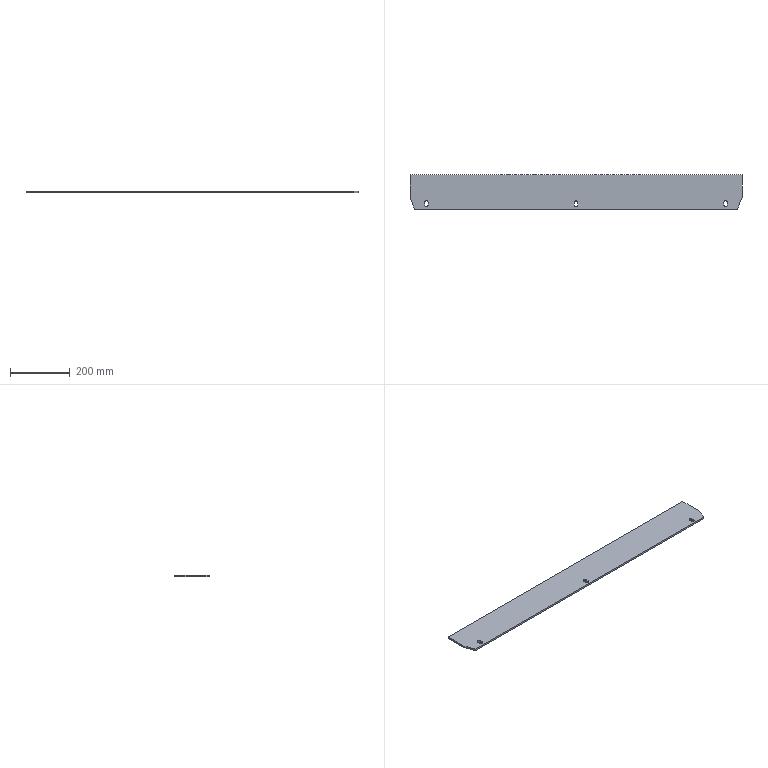Part | SolidWorks | features Extrusion 1, ICE 1 | 1 solid | 20 faces | box 1110 x 115 x 6 mm | volume 758807 mm3 | plane 14 | cylinder 6 | commonest cylinder face diameters 11 x6
STEP:
#1=CARTESIAN_POINT('',(-555.,57.5,0.));
#2=VERTEX_POINT('',#1);
#3=CARTESIAN_POINT('',(-555.,-17.5,0.));
#4=VERTEX_POINT('',#3);
#5=CARTESIAN_POINT('',(-555.,-57.5,0.));
#6=DIRECTION('',(0.,-1.,0.));
#7=VECTOR('',#6,1000.);
#8=LINE('',#5,#7);
#9=EDGE_CURVE('',#2,#4,#8,.T.);
#10=ORIENTED_EDGE('',*,*,#9,.T.);
#11=CARTESIAN_POINT('',(-555.,-17.5,6.));
#12=VERTEX_POINT('',#11);
#13=CARTESIAN_POINT('',(-555.,-17.5,0.));
#14=DIRECTION('',(0.,0.,1.));
#15=VECTOR('',#14,1000.);
#16=LINE('',#13,#15);
#17=EDGE_CURVE('',#4,#12,#16,.T.);
#18=ORIENTED_EDGE('',*,*,#17,.T.);
#19=CARTESIAN_POINT('',(-555.,57.5,6.));
#20=VERTEX_POINT('',#19);
#21=CARTESIAN_POINT('',(-555.,-57.5,6.));
#22=DIRECTION('',(0.,-1.,0.));
#23=VECTOR('',#22,1000.);
#24=LINE('',#21,#23);
#25=EDGE_CURVE('',#20,#12,#24,.T.);
#26=ORIENTED_EDGE('',*,*,#25,.F.);
#27=CARTESIAN_POINT('',(-555.,57.5,6.));
#28=DIRECTION('',(0.,0.,-1.));
#29=VECTOR('',#28,1000.);
#30=LINE('',#27,#29);
#31=EDGE_CURVE('',#20,#2,#30,.T.);
#32=ORIENTED_EDGE('',*,*,#31,.T.);
#33=EDGE_LOOP('',(#10,#18,#26,#32));
#34=FACE_OUTER_BOUND('',#33,.T.);
#35=CARTESIAN_POINT('',(-555.,-57.5,6.));
#36=DIRECTION('',(1.,0.,0.));
#37=DIRECTION('',(0.,0.,-1.));
#38=AXIS2_PLACEMENT_3D('',#35,#36,#37);
#39=PLANE('',#38);
#40=ADVANCED_FACE('',(#34),#39,.F.);
#41=CARTESIAN_POINT('',(-540.,-57.5,6.));
#42=VERTEX_POINT('',#41);
#43=CARTESIAN_POINT('',(540.,-57.5,6.));
#44=VERTEX_POINT('',#43);
#45=CARTESIAN_POINT('',(555.,-57.5,6.));
#46=DIRECTION('',(1.,0.,0.));
#47=VECTOR('',#46,1000.);
#48=LINE('',#45,#47);
#49=EDGE_CURVE('',#42,#44,#48,.T.);
#50=ORIENTED_EDGE('',*,*,#49,.F.);
#51=CARTESIAN_POINT('',(-540.,-57.5,0.));
#52=VERTEX_POINT('',#51);
#53=CARTESIAN_POINT('',(-540.,-57.5,0.));
#54=DIRECTION('',(0.,0.,1.));
#55=VECTOR('',#54,1000.);
#56=LINE('',#53,#55);
#57=EDGE_CURVE('',#52,#42,#56,.T.);
#58=ORIENTED_EDGE('',*,*,#57,.F.);
#59=CARTESIAN_POINT('',(540.,-57.5,0.));
#60=VERTEX_POINT('',#59);
#61=CARTESIAN_POINT('',(555.,-57.5,0.));
#62=DIRECTION('',(1.,0.,0.));
#63=VECTOR('',#62,1000.);
#64=LINE('',#61,#63);
#65=EDGE_CURVE('',#52,#60,#64,.T.);
#66=ORIENTED_EDGE('',*,*,#65,.T.);
#67=CARTESIAN_POINT('',(540.,-57.5,0.));
#68=DIRECTION('',(0.,0.,1.));
#69=VECTOR('',#68,1000.);
#70=LINE('',#67,#69);
#71=EDGE_CURVE('',#60,#44,#70,.T.);
#72=ORIENTED_EDGE('',*,*,#71,.T.);
#73=EDGE_LOOP('',(#50,#58,#66,#72));
#74=FACE_OUTER_BOUND('',#73,.T.);
#75=CARTESIAN_POINT('',(555.,-57.5,6.));
#76=DIRECTION('',(0.,1.,0.));
#77=DIRECTION('',(-1.,0.,0.));
#78=AXIS2_PLACEMENT_3D('',#75,#76,#77);
#79=PLANE('',#78);
#80=ADVANCED_FACE('',(#74),#79,.F.);
#81=CARTESIAN_POINT('',(555.,-17.5,6.));
#82=VERTEX_POINT('',#81);
#83=CARTESIAN_POINT('',(555.,57.5,6.));
#84=VERTEX_POINT('',#83);
#85=CARTESIAN_POINT('',(555.,-57.5,6.));
#86=DIRECTION('',(0.,1.,0.));
#87=VECTOR('',#86,1000.);
#88=LINE('',#85,#87);
#89=EDGE_CURVE('',#82,#84,#88,.T.);
#90=ORIENTED_EDGE('',*,*,#89,.F.);
#91=CARTESIAN_POINT('',(555.,-17.5,0.));
#92=VERTEX_POINT('',#91);
#93=CARTESIAN_POINT('',(555.,-17.5,0.));
#94=DIRECTION('',(0.,0.,1.));
#95=VECTOR('',#94,1000.);
#96=LINE('',#93,#95);
#97=EDGE_CURVE('',#92,#82,#96,.T.);
#98=ORIENTED_EDGE('',*,*,#97,.F.);
#99=CARTESIAN_POINT('',(555.,57.5,0.));
#100=VERTEX_POINT('',#99);
#101=CARTESIAN_POINT('',(555.,-57.5,0.));
#102=DIRECTION('',(0.,1.,0.));
#103=VECTOR('',#102,1000.);
#104=LINE('',#101,#103);
#105=EDGE_CURVE('',#92,#100,#104,.T.);
#106=ORIENTED_EDGE('',*,*,#105,.T.);
#107=CARTESIAN_POINT('',(555.,57.5,6.));
#108=DIRECTION('',(0.,0.,-1.));
#109=VECTOR('',#108,1000.);
#110=LINE('',#107,#109);
#111=EDGE_CURVE('',#84,#100,#110,.T.);
#112=ORIENTED_EDGE('',*,*,#111,.F.);
#113=EDGE_LOOP('',(#90,#98,#106,#112));
#114=FACE_OUTER_BOUND('',#113,.T.);
#115=CARTESIAN_POINT('',(555.,-57.5,6.));
#116=DIRECTION('',(-1.,0.,0.));
#117=DIRECTION('',(0.,0.,1.));
#118=AXIS2_PLACEMENT_3D('',#115,#116,#117);
#119=PLANE('',#118);
#120=ADVANCED_FACE('',(#114),#119,.F.);
#121=CARTESIAN_POINT('',(555.,57.5,0.));
#122=DIRECTION('',(-1.,0.,0.));
#123=VECTOR('',#122,1000.);
#124=LINE('',#121,#123);
#125=EDGE_CURVE('',#100,#2,#124,.T.);
#126=ORIENTED_EDGE('',*,*,#125,.T.);
#127=ORIENTED_EDGE('',*,*,#31,.F.);
#128=CARTESIAN_POINT('',(555.,57.5,6.));
#129=DIRECTION('',(-1.,0.,0.));
#130=VECTOR('',#129,1000.);
#131=LINE('',#128,#130);
#132=EDGE_CURVE('',#84,#20,#131,.T.);
#133=ORIENTED_EDGE('',*,*,#132,.F.);
#134=ORIENTED_EDGE('',*,*,#111,.T.);
#135=EDGE_LOOP('',(#126,#127,#133,#134));
#136=FACE_OUTER_BOUND('',#135,.T.);
#137=CARTESIAN_POINT('',(555.,57.5,6.));
#138=DIRECTION('',(0.,-1.,0.));
#139=DIRECTION('',(1.,0.,0.));
#140=AXIS2_PLACEMENT_3D('',#137,#138,#139);
#141=PLANE('',#140);
#142=ADVANCED_FACE('',(#136),#141,.F.);
#143=CARTESIAN_POINT('',(5.5,-35.,6.));
#144=VERTEX_POINT('',#143);
#145=CARTESIAN_POINT('',(-5.5,-35.,6.));
#146=VERTEX_POINT('',#145);
#147=CARTESIAN_POINT('',(0.,-35.,6.));
#148=DIRECTION('',(0.,0.,1.));
#149=DIRECTION('',(1.,0.,0.));
#150=AXIS2_PLACEMENT_3D('',#147,#148,#149);
#151=CIRCLE('',#150,5.5);
#152=EDGE_CURVE('',#144,#146,#151,.T.);
#153=ORIENTED_EDGE('',*,*,#152,.F.);
#154=CARTESIAN_POINT('',(5.5,-44.,6.));
#155=VERTEX_POINT('',#154);
#156=CARTESIAN_POINT('',(5.5,-35.,6.));
#157=DIRECTION('',(0.,1.,0.));
#158=VECTOR('',#157,1000.);
#159=LINE('',#156,#158);
#160=EDGE_CURVE('',#155,#144,#159,.T.);
#161=ORIENTED_EDGE('',*,*,#160,.F.);
#162=CARTESIAN_POINT('',(-5.5,-44.,6.));
#163=VERTEX_POINT('',#162);
#164=CARTESIAN_POINT('',(0.,-44.,6.));
#165=DIRECTION('',(0.,0.,1.));
#166=DIRECTION('',(1.,0.,0.));
#167=AXIS2_PLACEMENT_3D('',#164,#165,#166);
#168=CIRCLE('',#167,5.5);
#169=EDGE_CURVE('',#163,#155,#168,.T.);
#170=ORIENTED_EDGE('',*,*,#169,.F.);
#171=CARTESIAN_POINT('',(-5.5,-35.,6.));
#172=DIRECTION('',(0.,-1.,0.));
#173=VECTOR('',#172,1000.);
#174=LINE('',#171,#173);
#175=EDGE_CURVE('',#146,#163,#174,.T.);
#176=ORIENTED_EDGE('',*,*,#175,.F.);
#177=EDGE_LOOP('',(#153,#161,#170,#176));
#178=FACE_BOUND('',#177,.T.);
#179=CARTESIAN_POINT('',(494.5,-44.,6.));
#180=VERTEX_POINT('',#179);
#181=CARTESIAN_POINT('',(505.5,-44.,6.));
#182=VERTEX_POINT('',#181);
#183=CARTESIAN_POINT('',(500.,-44.,6.));
#184=DIRECTION('',(0.,0.,1.));
#185=DIRECTION('',(1.,0.,0.));
#186=AXIS2_PLACEMENT_3D('',#183,#184,#185);
#187=CIRCLE('',#186,5.5);
#188=EDGE_CURVE('',#180,#182,#187,.T.);
#189=ORIENTED_EDGE('',*,*,#188,.F.);
#190=CARTESIAN_POINT('',(494.5,-35.,6.));
#191=VERTEX_POINT('',#190);
#192=CARTESIAN_POINT('',(494.5,-44.,6.));
#193=DIRECTION('',(0.,-1.,0.));
#194=VECTOR('',#193,1000.);
#195=LINE('',#192,#194);
#196=EDGE_CURVE('',#191,#180,#195,.T.);
#197=ORIENTED_EDGE('',*,*,#196,.F.);
#198=CARTESIAN_POINT('',(505.5,-35.,6.));
#199=VERTEX_POINT('',#198);
#200=CARTESIAN_POINT('',(500.,-35.,6.));
#201=DIRECTION('',(0.,0.,1.));
#202=DIRECTION('',(1.,0.,0.));
#203=AXIS2_PLACEMENT_3D('',#200,#201,#202);
#204=CIRCLE('',#203,5.5);
#205=EDGE_CURVE('',#199,#191,#204,.T.);
#206=ORIENTED_EDGE('',*,*,#205,.F.);
#207=CARTESIAN_POINT('',(505.5,-44.,6.));
#208=DIRECTION('',(0.,1.,0.));
#209=VECTOR('',#208,1000.);
#210=LINE('',#207,#209);
#211=EDGE_CURVE('',#182,#199,#210,.T.);
#212=ORIENTED_EDGE('',*,*,#211,.F.);
#213=EDGE_LOOP('',(#189,#197,#206,#212));
#214=FACE_BOUND('',#213,.T.);
#215=CARTESIAN_POINT('',(-555.,-17.5,6.));
#216=DIRECTION('',(-0.3511,0.9363,0.));
#217=VECTOR('',#216,1000.);
#218=LINE('',#215,#217);
#219=EDGE_CURVE('',#42,#12,#218,.T.);
#220=ORIENTED_EDGE('',*,*,#219,.F.);
#221=ORIENTED_EDGE('',*,*,#49,.T.);
#222=CARTESIAN_POINT('',(555.,-17.5,6.));
#223=DIRECTION('',(-0.3511,-0.9363,0.));
#224=VECTOR('',#223,1000.);
#225=LINE('',#222,#224);
#226=EDGE_CURVE('',#82,#44,#225,.T.);
#227=ORIENTED_EDGE('',*,*,#226,.F.);
#228=ORIENTED_EDGE('',*,*,#89,.T.);
#229=ORIENTED_EDGE('',*,*,#132,.T.);
#230=ORIENTED_EDGE('',*,*,#25,.T.);
#231=EDGE_LOOP('',(#220,#221,#227,#228,#229,#230));
#232=FACE_OUTER_BOUND('',#231,.T.);
#233=CARTESIAN_POINT('',(-494.5,-35.,6.));
#234=VERTEX_POINT('',#233);
#235=CARTESIAN_POINT('',(-505.5,-35.,6.));
#236=VERTEX_POINT('',#235);
#237=CARTESIAN_POINT('',(-500.,-35.,6.));
#238=DIRECTION('',(0.,0.,1.));
#239=DIRECTION('',(1.,0.,0.));
#240=AXIS2_PLACEMENT_3D('',#237,#238,#239);
#241=CIRCLE('',#240,5.5);
#242=EDGE_CURVE('',#234,#236,#241,.T.);
#243=ORIENTED_EDGE('',*,*,#242,.F.);
#244=CARTESIAN_POINT('',(-494.5,-44.,6.));
#245=VERTEX_POINT('',#244);
#246=CARTESIAN_POINT('',(-494.5,-35.,6.));
#247=DIRECTION('',(0.,1.,0.));
#248=VECTOR('',#247,1000.);
#249=LINE('',#246,#248);
#250=EDGE_CURVE('',#245,#234,#249,.T.);
#251=ORIENTED_EDGE('',*,*,#250,.F.);
#252=CARTESIAN_POINT('',(-505.5,-44.,6.));
#253=VERTEX_POINT('',#252);
#254=CARTESIAN_POINT('',(-500.,-44.,6.));
#255=DIRECTION('',(0.,0.,1.));
#256=DIRECTION('',(1.,0.,0.));
#257=AXIS2_PLACEMENT_3D('',#254,#255,#256);
#258=CIRCLE('',#257,5.5);
#259=EDGE_CURVE('',#253,#245,#258,.T.);
#260=ORIENTED_EDGE('',*,*,#259,.F.);
#261=CARTESIAN_POINT('',(-505.5,-35.,6.));
#262=DIRECTION('',(0.,-1.,0.));
#263=VECTOR('',#262,1000.);
#264=LINE('',#261,#263);
#265=EDGE_CURVE('',#236,#253,#264,.T.);
#266=ORIENTED_EDGE('',*,*,#265,.F.);
#267=EDGE_LOOP('',(#243,#251,#260,#266));
#268=FACE_BOUND('',#267,.T.);
#269=CARTESIAN_POINT('',(0.,0.,6.));
#270=DIRECTION('',(0.,0.,1.));
#271=DIRECTION('',(1.,0.,0.));
#272=AXIS2_PLACEMENT_3D('',#269,#270,#271);
#273=PLANE('',#272);
#274=ADVANCED_FACE('',(#178,#214,#232,#268),#273,.T.);
#275=CARTESIAN_POINT('',(5.5,-44.,0.));
#276=VERTEX_POINT('',#275);
#277=CARTESIAN_POINT('',(5.5,-35.,0.));
#278=VERTEX_POINT('',#277);
#279=CARTESIAN_POINT('',(5.5,-35.,0.));
#280=DIRECTION('',(0.,1.,0.));
#281=VECTOR('',#280,1000.);
#282=LINE('',#279,#281);
#283=EDGE_CURVE('',#276,#278,#282,.T.);
#284=ORIENTED_EDGE('',*,*,#283,.T.);
#285=CARTESIAN_POINT('',(-5.5,-35.,0.));
#286=VERTEX_POINT('',#285);
#287=CARTESIAN_POINT('',(0.,-35.,0.));
#288=DIRECTION('',(0.,0.,1.));
#289=DIRECTION('',(1.,0.,0.));
#290=AXIS2_PLACEMENT_3D('',#287,#288,#289);
#291=CIRCLE('',#290,5.5);
#292=EDGE_CURVE('',#278,#286,#291,.T.);
#293=ORIENTED_EDGE('',*,*,#292,.T.);
#294=CARTESIAN_POINT('',(-5.5,-44.,0.));
#295=VERTEX_POINT('',#294);
#296=CARTESIAN_POINT('',(-5.5,-35.,0.));
#297=DIRECTION('',(0.,-1.,0.));
#298=VECTOR('',#297,1000.);
#299=LINE('',#296,#298);
#300=EDGE_CURVE('',#286,#295,#299,.T.);
#301=ORIENTED_EDGE('',*,*,#300,.T.);
#302=CARTESIAN_POINT('',(0.,-44.,0.));
#303=DIRECTION('',(0.,0.,1.));
#304=DIRECTION('',(1.,0.,0.));
#305=AXIS2_PLACEMENT_3D('',#302,#303,#304);
#306=CIRCLE('',#305,5.5);
#307=EDGE_CURVE('',#295,#276,#306,.T.);
#308=ORIENTED_EDGE('',*,*,#307,.T.);
#309=EDGE_LOOP('',(#284,#293,#301,#308));
#310=FACE_BOUND('',#309,.T.);
#311=CARTESIAN_POINT('',(494.5,-35.,0.));
#312=VERTEX_POINT('',#311);
#313=CARTESIAN_POINT('',(494.5,-44.,0.));
#314=VERTEX_POINT('',#313);
#315=CARTESIAN_POINT('',(494.5,-44.,0.));
#316=DIRECTION('',(0.,-1.,0.));
#317=VECTOR('',#316,1000.);
#318=LINE('',#315,#317);
#319=EDGE_CURVE('',#312,#314,#318,.T.);
#320=ORIENTED_EDGE('',*,*,#319,.T.);
#321=CARTESIAN_POINT('',(505.5,-44.,0.));
#322=VERTEX_POINT('',#321);
#323=CARTESIAN_POINT('',(500.,-44.,0.));
#324=DIRECTION('',(0.,0.,1.));
#325=DIRECTION('',(1.,0.,0.));
#326=AXIS2_PLACEMENT_3D('',#323,#324,#325);
#327=CIRCLE('',#326,5.5);
#328=EDGE_CURVE('',#314,#322,#327,.T.);
#329=ORIENTED_EDGE('',*,*,#328,.T.);
#330=CARTESIAN_POINT('',(505.5,-35.,0.));
#331=VERTEX_POINT('',#330);
#332=CARTESIAN_POINT('',(505.5,-44.,0.));
#333=DIRECTION('',(0.,1.,0.));
#334=VECTOR('',#333,1000.);
#335=LINE('',#332,#334);
#336=EDGE_CURVE('',#322,#331,#335,.T.);
#337=ORIENTED_EDGE('',*,*,#336,.T.);
#338=CARTESIAN_POINT('',(500.,-35.,0.));
#339=DIRECTION('',(0.,0.,1.));
#340=DIRECTION('',(1.,0.,0.));
#341=AXIS2_PLACEMENT_3D('',#338,#339,#340);
#342=CIRCLE('',#341,5.5);
#343=EDGE_CURVE('',#331,#312,#342,.T.);
#344=ORIENTED_EDGE('',*,*,#343,.T.);
#345=EDGE_LOOP('',(#320,#329,#337,#344));
#346=FACE_BOUND('',#345,.T.);
#347=CARTESIAN_POINT('',(-494.5,-44.,0.));
#348=VERTEX_POINT('',#347);
#349=CARTESIAN_POINT('',(-494.5,-35.,0.));
#350=VERTEX_POINT('',#349);
#351=CARTESIAN_POINT('',(-494.5,-35.,0.));
#352=DIRECTION('',(0.,1.,0.));
#353=VECTOR('',#352,1000.);
#354=LINE('',#351,#353);
#355=EDGE_CURVE('',#348,#350,#354,.T.);
#356=ORIENTED_EDGE('',*,*,#355,.T.);
#357=CARTESIAN_POINT('',(-505.5,-35.,0.));
#358=VERTEX_POINT('',#357);
#359=CARTESIAN_POINT('',(-500.,-35.,0.));
#360=DIRECTION('',(0.,0.,1.));
#361=DIRECTION('',(1.,0.,0.));
#362=AXIS2_PLACEMENT_3D('',#359,#360,#361);
#363=CIRCLE('',#362,5.5);
#364=EDGE_CURVE('',#350,#358,#363,.T.);
#365=ORIENTED_EDGE('',*,*,#364,.T.);
#366=CARTESIAN_POINT('',(-505.5,-44.,0.));
#367=VERTEX_POINT('',#366);
#368=CARTESIAN_POINT('',(-505.5,-35.,0.));
#369=DIRECTION('',(0.,-1.,0.));
#370=VECTOR('',#369,1000.);
#371=LINE('',#368,#370);
#372=EDGE_CURVE('',#358,#367,#371,.T.);
#373=ORIENTED_EDGE('',*,*,#372,.T.);
#374=CARTESIAN_POINT('',(-500.,-44.,0.));
#375=DIRECTION('',(0.,0.,1.));
#376=DIRECTION('',(1.,0.,0.));
#377=AXIS2_PLACEMENT_3D('',#374,#375,#376);
#378=CIRCLE('',#377,5.5);
#379=EDGE_CURVE('',#367,#348,#378,.T.);
#380=ORIENTED_EDGE('',*,*,#379,.T.);
#381=EDGE_LOOP('',(#356,#365,#373,#380));
#382=FACE_BOUND('',#381,.T.);
#383=ORIENTED_EDGE('',*,*,#65,.F.);
#384=CARTESIAN_POINT('',(-555.,-17.5,0.));
#385=DIRECTION('',(-0.3511,0.9363,0.));
#386=VECTOR('',#385,1000.);
#387=LINE('',#384,#386);
#388=EDGE_CURVE('',#52,#4,#387,.T.);
#389=ORIENTED_EDGE('',*,*,#388,.T.);
#390=ORIENTED_EDGE('',*,*,#9,.F.);
#391=ORIENTED_EDGE('',*,*,#125,.F.);
#392=ORIENTED_EDGE('',*,*,#105,.F.);
#393=CARTESIAN_POINT('',(555.,-17.5,0.));
#394=DIRECTION('',(-0.3511,-0.9363,0.));
#395=VECTOR('',#394,1000.);
#396=LINE('',#393,#395);
#397=EDGE_CURVE('',#92,#60,#396,.T.);
#398=ORIENTED_EDGE('',*,*,#397,.T.);
#399=EDGE_LOOP('',(#383,#389,#390,#391,#392,#398));
#400=FACE_OUTER_BOUND('',#399,.T.);
#401=CARTESIAN_POINT('',(0.,0.,0.));
#402=DIRECTION('',(0.,0.,1.));
#403=DIRECTION('',(1.,0.,0.));
#404=AXIS2_PLACEMENT_3D('',#401,#402,#403);
#405=PLANE('',#404);
#406=ADVANCED_FACE('',(#310,#346,#382,#400),#405,.F.);
#407=ORIENTED_EDGE('',*,*,#242,.T.);
#408=CARTESIAN_POINT('',(-505.5,-35.,0.));
#409=DIRECTION('',(0.,0.,1.));
#410=VECTOR('',#409,1000.);
#411=LINE('',#408,#410);
#412=EDGE_CURVE('',#358,#236,#411,.T.);
#413=ORIENTED_EDGE('',*,*,#412,.F.);
#414=ORIENTED_EDGE('',*,*,#364,.F.);
#415=CARTESIAN_POINT('',(-494.5,-35.,0.));
#416=DIRECTION('',(0.,0.,1.));
#417=VECTOR('',#416,1000.);
#418=LINE('',#415,#417);
#419=EDGE_CURVE('',#350,#234,#418,.T.);
#420=ORIENTED_EDGE('',*,*,#419,.T.);
#421=EDGE_LOOP('',(#407,#413,#414,#420));
#422=FACE_OUTER_BOUND('',#421,.T.);
#423=CARTESIAN_POINT('',(-500.,-35.,0.));
#424=DIRECTION('',(0.,0.,1.));
#425=DIRECTION('',(1.,0.,0.));
#426=AXIS2_PLACEMENT_3D('',#423,#424,#425);
#427=CYLINDRICAL_SURFACE('',#426,5.5);
#428=ADVANCED_FACE('',(#422),#427,.F.);
#429=ORIENTED_EDGE('',*,*,#250,.T.);
#430=ORIENTED_EDGE('',*,*,#419,.F.);
#431=ORIENTED_EDGE('',*,*,#355,.F.);
#432=CARTESIAN_POINT('',(-494.5,-44.,0.));
#433=DIRECTION('',(0.,0.,1.));
#434=VECTOR('',#433,1000.);
#435=LINE('',#432,#434);
#436=EDGE_CURVE('',#348,#245,#435,.T.);
#437=ORIENTED_EDGE('',*,*,#436,.T.);
#438=EDGE_LOOP('',(#429,#430,#431,#437));
#439=FACE_OUTER_BOUND('',#438,.T.);
#440=CARTESIAN_POINT('',(-494.5,-35.,0.));
#441=DIRECTION('',(1.,0.,0.));
#442=DIRECTION('',(0.,0.,-1.));
#443=AXIS2_PLACEMENT_3D('',#440,#441,#442);
#444=PLANE('',#443);
#445=ADVANCED_FACE('',(#439),#444,.F.);
#446=ORIENTED_EDGE('',*,*,#259,.T.);
#447=ORIENTED_EDGE('',*,*,#436,.F.);
#448=ORIENTED_EDGE('',*,*,#379,.F.);
#449=CARTESIAN_POINT('',(-505.5,-44.,0.));
#450=DIRECTION('',(0.,0.,1.));
#451=VECTOR('',#450,1000.);
#452=LINE('',#449,#451);
#453=EDGE_CURVE('',#367,#253,#452,.T.);
#454=ORIENTED_EDGE('',*,*,#453,.T.);
#455=EDGE_LOOP('',(#446,#447,#448,#454));
#456=FACE_OUTER_BOUND('',#455,.T.);
#457=CARTESIAN_POINT('',(-500.,-44.,0.));
#458=DIRECTION('',(0.,0.,1.));
#459=DIRECTION('',(1.,0.,0.));
#460=AXIS2_PLACEMENT_3D('',#457,#458,#459);
#461=CYLINDRICAL_SURFACE('',#460,5.5);
#462=ADVANCED_FACE('',(#456),#461,.F.);
#463=ORIENTED_EDGE('',*,*,#265,.T.);
#464=ORIENTED_EDGE('',*,*,#453,.F.);
#465=ORIENTED_EDGE('',*,*,#372,.F.);
#466=ORIENTED_EDGE('',*,*,#412,.T.);
#467=EDGE_LOOP('',(#463,#464,#465,#466));
#468=FACE_OUTER_BOUND('',#467,.T.);
#469=CARTESIAN_POINT('',(-505.5,-35.,0.));
#470=DIRECTION('',(-1.,0.,0.));
#471=DIRECTION('',(0.,0.,1.));
#472=AXIS2_PLACEMENT_3D('',#469,#470,#471);
#473=PLANE('',#472);
#474=ADVANCED_FACE('',(#468),#473,.F.);
#475=ORIENTED_EDGE('',*,*,#226,.T.);
#476=ORIENTED_EDGE('',*,*,#71,.F.);
#477=ORIENTED_EDGE('',*,*,#397,.F.);
#478=ORIENTED_EDGE('',*,*,#97,.T.);
#479=EDGE_LOOP('',(#475,#476,#477,#478));
#480=FACE_OUTER_BOUND('',#479,.T.);
#481=CARTESIAN_POINT('',(555.,-17.5,0.));
#482=DIRECTION('',(-0.9363,0.3511,0.));
#483=DIRECTION('',(-0.3511,-0.9363,0.));
#484=AXIS2_PLACEMENT_3D('',#481,#482,#483);
#485=PLANE('',#484);
#486=ADVANCED_FACE('',(#480),#485,.F.);
#487=ORIENTED_EDGE('',*,*,#219,.T.);
#488=ORIENTED_EDGE('',*,*,#17,.F.);
#489=ORIENTED_EDGE('',*,*,#388,.F.);
#490=ORIENTED_EDGE('',*,*,#57,.T.);
#491=EDGE_LOOP('',(#487,#488,#489,#490));
#492=FACE_OUTER_BOUND('',#491,.T.);
#493=CARTESIAN_POINT('',(-555.,-17.5,0.));
#494=DIRECTION('',(0.9363,0.3511,0.));
#495=DIRECTION('',(-0.3511,0.9363,0.));
#496=AXIS2_PLACEMENT_3D('',#493,#494,#495);
#497=PLANE('',#496);
#498=ADVANCED_FACE('',(#492),#497,.F.);
#499=ORIENTED_EDGE('',*,*,#188,.T.);
#500=CARTESIAN_POINT('',(505.5,-44.,0.));
#501=DIRECTION('',(0.,0.,1.));
#502=VECTOR('',#501,1000.);
#503=LINE('',#500,#502);
#504=EDGE_CURVE('',#322,#182,#503,.T.);
#505=ORIENTED_EDGE('',*,*,#504,.F.);
#506=ORIENTED_EDGE('',*,*,#328,.F.);
#507=CARTESIAN_POINT('',(494.5,-44.,0.));
#508=DIRECTION('',(0.,0.,1.));
#509=VECTOR('',#508,1000.);
#510=LINE('',#507,#509);
#511=EDGE_CURVE('',#314,#180,#510,.T.);
#512=ORIENTED_EDGE('',*,*,#511,.T.);
#513=EDGE_LOOP('',(#499,#505,#506,#512));
#514=FACE_OUTER_BOUND('',#513,.T.);
#515=CARTESIAN_POINT('',(500.,-44.,0.));
#516=DIRECTION('',(0.,0.,1.));
#517=DIRECTION('',(1.,0.,0.));
#518=AXIS2_PLACEMENT_3D('',#515,#516,#517);
#519=CYLINDRICAL_SURFACE('',#518,5.5);
#520=ADVANCED_FACE('',(#514),#519,.F.);
#521=ORIENTED_EDGE('',*,*,#196,.T.);
#522=ORIENTED_EDGE('',*,*,#511,.F.);
#523=ORIENTED_EDGE('',*,*,#319,.F.);
#524=CARTESIAN_POINT('',(494.5,-35.,0.));
#525=DIRECTION('',(0.,0.,1.));
#526=VECTOR('',#525,1000.);
#527=LINE('',#524,#526);
#528=EDGE_CURVE('',#312,#191,#527,.T.);
#529=ORIENTED_EDGE('',*,*,#528,.T.);
#530=EDGE_LOOP('',(#521,#522,#523,#529));
#531=FACE_OUTER_BOUND('',#530,.T.);
#532=CARTESIAN_POINT('',(494.5,-44.,0.));
#533=DIRECTION('',(-1.,0.,0.));
#534=DIRECTION('',(0.,0.,1.));
#535=AXIS2_PLACEMENT_3D('',#532,#533,#534);
#536=PLANE('',#535);
#537=ADVANCED_FACE('',(#531),#536,.F.);
#538=ORIENTED_EDGE('',*,*,#205,.T.);
#539=ORIENTED_EDGE('',*,*,#528,.F.);
#540=ORIENTED_EDGE('',*,*,#343,.F.);
#541=CARTESIAN_POINT('',(505.5,-35.,0.));
#542=DIRECTION('',(0.,0.,1.));
#543=VECTOR('',#542,1000.);
#544=LINE('',#541,#543);
#545=EDGE_CURVE('',#331,#199,#544,.T.);
#546=ORIENTED_EDGE('',*,*,#545,.T.);
#547=EDGE_LOOP('',(#538,#539,#540,#546));
#548=FACE_OUTER_BOUND('',#547,.T.);
#549=CARTESIAN_POINT('',(500.,-35.,0.));
#550=DIRECTION('',(0.,0.,1.));
#551=DIRECTION('',(1.,0.,0.));
#552=AXIS2_PLACEMENT_3D('',#549,#550,#551);
#553=CYLINDRICAL_SURFACE('',#552,5.5);
#554=ADVANCED_FACE('',(#548),#553,.F.);
#555=ORIENTED_EDGE('',*,*,#211,.T.);
#556=ORIENTED_EDGE('',*,*,#545,.F.);
#557=ORIENTED_EDGE('',*,*,#336,.F.);
#558=ORIENTED_EDGE('',*,*,#504,.T.);
#559=EDGE_LOOP('',(#555,#556,#557,#558));
#560=FACE_OUTER_BOUND('',#559,.T.);
#561=CARTESIAN_POINT('',(505.5,-44.,0.));
#562=DIRECTION('',(1.,0.,0.));
#563=DIRECTION('',(0.,0.,-1.));
#564=AXIS2_PLACEMENT_3D('',#561,#562,#563);
#565=PLANE('',#564);
#566=ADVANCED_FACE('',(#560),#565,.F.);
#567=ORIENTED_EDGE('',*,*,#152,.T.);
#568=CARTESIAN_POINT('',(-5.5,-35.,0.));
#569=DIRECTION('',(0.,0.,1.));
#570=VECTOR('',#569,1000.);
#571=LINE('',#568,#570);
#572=EDGE_CURVE('',#286,#146,#571,.T.);
#573=ORIENTED_EDGE('',*,*,#572,.F.);
#574=ORIENTED_EDGE('',*,*,#292,.F.);
#575=CARTESIAN_POINT('',(5.5,-35.,0.));
#576=DIRECTION('',(0.,0.,1.));
#577=VECTOR('',#576,1000.);
#578=LINE('',#575,#577);
#579=EDGE_CURVE('',#278,#144,#578,.T.);
#580=ORIENTED_EDGE('',*,*,#579,.T.);
#581=EDGE_LOOP('',(#567,#573,#574,#580));
#582=FACE_OUTER_BOUND('',#581,.T.);
#583=CARTESIAN_POINT('',(0.,-35.,0.));
#584=DIRECTION('',(0.,0.,1.));
#585=DIRECTION('',(1.,0.,0.));
#586=AXIS2_PLACEMENT_3D('',#583,#584,#585);
#587=CYLINDRICAL_SURFACE('',#586,5.5);
#588=ADVANCED_FACE('',(#582),#587,.F.);
#589=ORIENTED_EDGE('',*,*,#160,.T.);
#590=ORIENTED_EDGE('',*,*,#579,.F.);
#591=ORIENTED_EDGE('',*,*,#283,.F.);
#592=CARTESIAN_POINT('',(5.5,-44.,0.));
#593=DIRECTION('',(0.,0.,1.));
#594=VECTOR('',#593,1000.);
#595=LINE('',#592,#594);
#596=EDGE_CURVE('',#276,#155,#595,.T.);
#597=ORIENTED_EDGE('',*,*,#596,.T.);
#598=EDGE_LOOP('',(#589,#590,#591,#597));
#599=FACE_OUTER_BOUND('',#598,.T.);
#600=CARTESIAN_POINT('',(5.5,-35.,0.));
#601=DIRECTION('',(1.,0.,0.));
#602=DIRECTION('',(0.,1.,0.));
#603=AXIS2_PLACEMENT_3D('',#600,#601,#602);
#604=PLANE('',#603);
#605=ADVANCED_FACE('',(#599),#604,.F.);
#606=ORIENTED_EDGE('',*,*,#169,.T.);
#607=ORIENTED_EDGE('',*,*,#596,.F.);
#608=ORIENTED_EDGE('',*,*,#307,.F.);
#609=CARTESIAN_POINT('',(-5.5,-44.,0.));
#610=DIRECTION('',(0.,0.,1.));
#611=VECTOR('',#610,1000.);
#612=LINE('',#609,#611);
#613=EDGE_CURVE('',#295,#163,#612,.T.);
#614=ORIENTED_EDGE('',*,*,#613,.T.);
#615=EDGE_LOOP('',(#606,#607,#608,#614));
#616=FACE_OUTER_BOUND('',#615,.T.);
#617=CARTESIAN_POINT('',(0.,-44.,0.));
#618=DIRECTION('',(0.,0.,1.));
#619=DIRECTION('',(1.,0.,0.));
#620=AXIS2_PLACEMENT_3D('',#617,#618,#619);
#621=CYLINDRICAL_SURFACE('',#620,5.5);
#622=ADVANCED_FACE('',(#616),#621,.F.);
#623=ORIENTED_EDGE('',*,*,#175,.T.);
#624=ORIENTED_EDGE('',*,*,#613,.F.);
#625=ORIENTED_EDGE('',*,*,#300,.F.);
#626=ORIENTED_EDGE('',*,*,#572,.T.);
#627=EDGE_LOOP('',(#623,#624,#625,#626));
#628=FACE_OUTER_BOUND('',#627,.T.);
#629=CARTESIAN_POINT('',(-5.5,-35.,0.));
#630=DIRECTION('',(-1.,0.,0.));
#631=DIRECTION('',(0.,-1.,0.));
#632=AXIS2_PLACEMENT_3D('',#629,#630,#631);
#633=PLANE('',#632);
#634=ADVANCED_FACE('',(#628),#633,.F.);
#635=CLOSED_SHELL('',(#40,#80,#120,#142,#274,#406,#428,#445,#462,#474,#486,#498,#520,#537,#554,#566,#588,#605,#622,#634));
#636=MANIFOLD_SOLID_BREP('',#635);
#637=CARTESIAN_POINT('',(0.,0.,0.));
#638=DIRECTION('',(0.,0.,1.));
#639=DIRECTION('',(1.,0.,0.));
#640=AXIS2_PLACEMENT_3D('',#637,#638,#639);
#641=(LENGTH_UNIT()NAMED_UNIT(*)SI_UNIT(.MILLI.,.METRE.));
#642=UNCERTAINTY_MEASURE_WITH_UNIT(LENGTH_MEASURE(0.00001),#641,'','');
#643=(NAMED_UNIT(*)PLANE_ANGLE_UNIT()SI_UNIT($,.RADIAN.));
#644=(NAMED_UNIT(*)SI_UNIT($,.STERADIAN.)SOLID_ANGLE_UNIT());
#645=(GEOMETRIC_REPRESENTATION_CONTEXT(3)GLOBAL_UNCERTAINTY_ASSIGNED_CONTEXT((#642))GLOBAL_UNIT_ASSIGNED_CONTEXT((#641,#643,#644))REPRESENTATION_CONTEXT('',''));
#646=ADVANCED_BREP_SHAPE_REPRESENTATION('',(#636,#640),#645);